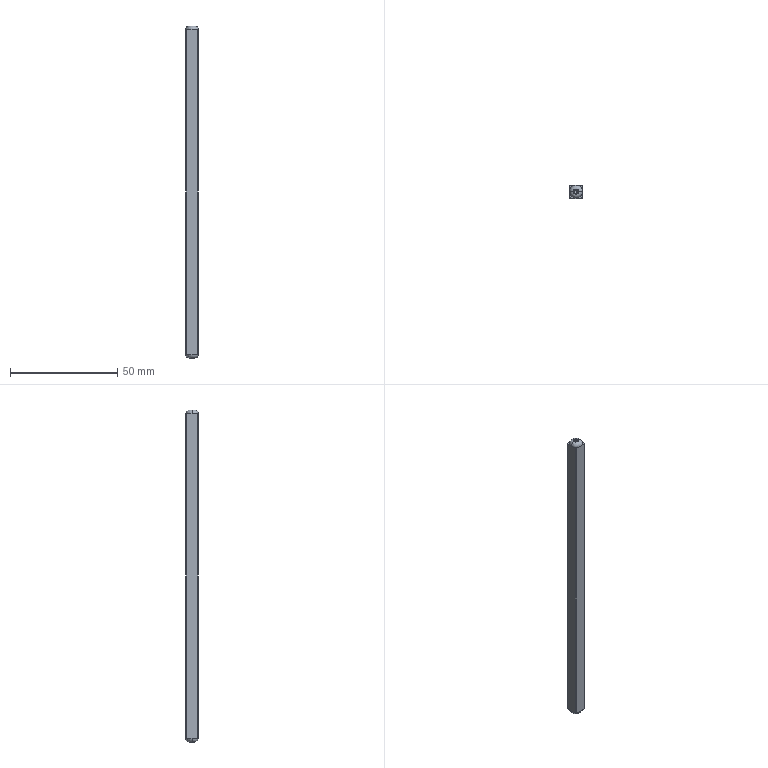Part | NX | features BREP 1 | 1 solid | 34 faces | box 6 x 6 x 155 mm | volume 5484 mm3 | plane 14 | cone 8 | cylinder 8 | torus 4 | commonest cylinder face diameters 1.5 x4 8 x4
STEP:
#1=CARTESIAN_POINT('',(0.75,0.,-77.25));
#2=VERTEX_POINT('',#1);
#3=CARTESIAN_POINT('',(1.,0.,-77.5));
#4=VERTEX_POINT('',#3);
#5=CARTESIAN_POINT('',(1.,0.,-77.5));
#6=DIRECTION('',(0.7071,0.,-0.7071));
#7=VECTOR('',#6,1000.);
#8=LINE('',#5,#7);
#9=EDGE_CURVE('',#2,#4,#8,.T.);
#10=ORIENTED_EDGE('',*,*,#9,.F.);
#11=CARTESIAN_POINT('',(-0.75,0.,-77.25));
#12=VERTEX_POINT('',#11);
#13=CARTESIAN_POINT('',(0.,0.,-77.25));
#14=DIRECTION('',(0.,0.,-1.));
#15=DIRECTION('',(-1.,0.,0.));
#16=AXIS2_PLACEMENT_3D('',#13,#14,#15);
#17=CIRCLE('',#16,0.75);
#18=EDGE_CURVE('',#12,#2,#17,.T.);
#19=ORIENTED_EDGE('',*,*,#18,.F.);
#20=CARTESIAN_POINT('',(-1.,0.,-77.5));
#21=VERTEX_POINT('',#20);
#22=CARTESIAN_POINT('',(-1.,0.,-77.5));
#23=DIRECTION('',(-0.7071,0.,-0.7071));
#24=VECTOR('',#23,1000.);
#25=LINE('',#22,#24);
#26=EDGE_CURVE('',#12,#21,#25,.T.);
#27=ORIENTED_EDGE('',*,*,#26,.T.);
#28=CARTESIAN_POINT('',(0.,0.,-77.5));
#29=DIRECTION('',(0.,0.,-1.));
#30=DIRECTION('',(-1.,0.,0.));
#31=AXIS2_PLACEMENT_3D('',#28,#29,#30);
#32=CIRCLE('',#31,1.);
#33=EDGE_CURVE('',#21,#4,#32,.T.);
#34=ORIENTED_EDGE('',*,*,#33,.T.);
#35=EDGE_LOOP('',(#10,#19,#27,#34));
#36=FACE_BOUND('',#35,.T.);
#37=CARTESIAN_POINT('',(0.,0.,-77.5));
#38=DIRECTION('',(0.,0.,-1.));
#39=DIRECTION('',(-1.,0.,0.));
#40=AXIS2_PLACEMENT_3D('',#37,#38,#39);
#41=CONICAL_SURFACE('',#40,1.,0.7854);
#42=ADVANCED_FACE('',(#36),#41,.F.);
#43=CARTESIAN_POINT('',(0.75,0.,-74.5));
#44=VERTEX_POINT('',#43);
#45=CARTESIAN_POINT('',(0.75,0.,-77.5));
#46=DIRECTION('',(0.,0.,-1.));
#47=VECTOR('',#46,1000.);
#48=LINE('',#45,#47);
#49=EDGE_CURVE('',#44,#2,#48,.T.);
#50=ORIENTED_EDGE('',*,*,#49,.F.);
#51=CARTESIAN_POINT('',(-0.75,0.,-74.5));
#52=VERTEX_POINT('',#51);
#53=CARTESIAN_POINT('',(0.,0.,-74.5));
#54=DIRECTION('',(0.,0.,-1.));
#55=DIRECTION('',(-1.,0.,0.));
#56=AXIS2_PLACEMENT_3D('',#53,#54,#55);
#57=CIRCLE('',#56,0.75);
#58=EDGE_CURVE('',#52,#44,#57,.T.);
#59=ORIENTED_EDGE('',*,*,#58,.F.);
#60=CARTESIAN_POINT('',(-0.75,0.,-77.5));
#61=DIRECTION('',(0.,0.,-1.));
#62=VECTOR('',#61,1000.);
#63=LINE('',#60,#62);
#64=EDGE_CURVE('',#52,#12,#63,.T.);
#65=ORIENTED_EDGE('',*,*,#64,.T.);
#66=ORIENTED_EDGE('',*,*,#18,.T.);
#67=EDGE_LOOP('',(#50,#59,#65,#66));
#68=FACE_BOUND('',#67,.T.);
#69=CARTESIAN_POINT('',(0.,0.,-77.5));
#70=DIRECTION('',(0.,0.,-1.));
#71=DIRECTION('',(-1.,0.,0.));
#72=AXIS2_PLACEMENT_3D('',#69,#70,#71);
#73=CYLINDRICAL_SURFACE('',#72,0.75);
#74=ADVANCED_FACE('',(#68),#73,.F.);
#75=CARTESIAN_POINT('',(0.,0.,-74.049));
#76=VERTEX_POINT('',#75);
#77=CARTESIAN_POINT('',(0.75,0.,-74.5));
#78=DIRECTION('',(0.8572,0.,-0.515));
#79=VECTOR('',#78,1000.);
#80=LINE('',#77,#79);
#81=EDGE_CURVE('',#44,#76,#80,.F.);
#82=ORIENTED_EDGE('',*,*,#81,.T.);
#83=CARTESIAN_POINT('',(-0.75,0.,-74.5));
#84=DIRECTION('',(-0.8572,0.,-0.515));
#85=VECTOR('',#84,1000.);
#86=LINE('',#83,#85);
#87=EDGE_CURVE('',#52,#76,#86,.F.);
#88=ORIENTED_EDGE('',*,*,#87,.F.);
#89=ORIENTED_EDGE('',*,*,#58,.T.);
#90=EDGE_LOOP('',(#82,#88,#89));
#91=FACE_BOUND('',#90,.T.);
#92=CARTESIAN_POINT('',(0.,0.,-74.5));
#93=DIRECTION('',(0.,0.,-1.));
#94=DIRECTION('',(-1.,0.,0.));
#95=AXIS2_PLACEMENT_3D('',#92,#93,#94);
#96=CONICAL_SURFACE('',#95,0.75,1.03);
#97=ADVANCED_FACE('',(#91),#96,.F.);
#98=CARTESIAN_POINT('',(-1.,0.,77.5));
#99=VERTEX_POINT('',#98);
#100=CARTESIAN_POINT('',(-0.75,0.,77.25));
#101=VERTEX_POINT('',#100);
#102=CARTESIAN_POINT('',(-1.,0.,77.5));
#103=DIRECTION('',(-0.7071,0.,0.7071));
#104=VECTOR('',#103,1000.);
#105=LINE('',#102,#104);
#106=EDGE_CURVE('',#99,#101,#105,.F.);
#107=ORIENTED_EDGE('',*,*,#106,.T.);
#108=CARTESIAN_POINT('',(0.75,0.,77.25));
#109=VERTEX_POINT('',#108);
#110=CARTESIAN_POINT('',(0.,0.,77.25));
#111=DIRECTION('',(0.,0.,1.));
#112=DIRECTION('',(1.,0.,0.));
#113=AXIS2_PLACEMENT_3D('',#110,#111,#112);
#114=CIRCLE('',#113,0.75);
#115=EDGE_CURVE('',#109,#101,#114,.T.);
#116=ORIENTED_EDGE('',*,*,#115,.F.);
#117=CARTESIAN_POINT('',(1.,0.,77.5));
#118=VERTEX_POINT('',#117);
#119=CARTESIAN_POINT('',(1.,0.,77.5));
#120=DIRECTION('',(0.7071,0.,0.7071));
#121=VECTOR('',#120,1000.);
#122=LINE('',#119,#121);
#123=EDGE_CURVE('',#118,#109,#122,.F.);
#124=ORIENTED_EDGE('',*,*,#123,.F.);
#125=CARTESIAN_POINT('',(0.,0.,77.5));
#126=DIRECTION('',(0.,0.,1.));
#127=DIRECTION('',(1.,0.,0.));
#128=AXIS2_PLACEMENT_3D('',#125,#126,#127);
#129=CIRCLE('',#128,1.);
#130=EDGE_CURVE('',#118,#99,#129,.T.);
#131=ORIENTED_EDGE('',*,*,#130,.T.);
#132=EDGE_LOOP('',(#107,#116,#124,#131));
#133=FACE_BOUND('',#132,.T.);
#134=CARTESIAN_POINT('',(0.,0.,77.5));
#135=DIRECTION('',(0.,0.,1.));
#136=DIRECTION('',(1.,0.,0.));
#137=AXIS2_PLACEMENT_3D('',#134,#135,#136);
#138=CONICAL_SURFACE('',#137,1.,0.7854);
#139=ADVANCED_FACE('',(#133),#138,.F.);
#140=CARTESIAN_POINT('',(-0.75,0.,74.5));
#141=VERTEX_POINT('',#140);
#142=CARTESIAN_POINT('',(-0.75,0.,77.5));
#143=DIRECTION('',(0.,0.,1.));
#144=VECTOR('',#143,1000.);
#145=LINE('',#142,#144);
#146=EDGE_CURVE('',#101,#141,#145,.F.);
#147=ORIENTED_EDGE('',*,*,#146,.T.);
#148=CARTESIAN_POINT('',(0.75,0.,74.5));
#149=VERTEX_POINT('',#148);
#150=CARTESIAN_POINT('',(0.,0.,74.5));
#151=DIRECTION('',(0.,0.,1.));
#152=DIRECTION('',(1.,0.,0.));
#153=AXIS2_PLACEMENT_3D('',#150,#151,#152);
#154=CIRCLE('',#153,0.75);
#155=EDGE_CURVE('',#149,#141,#154,.T.);
#156=ORIENTED_EDGE('',*,*,#155,.F.);
#157=CARTESIAN_POINT('',(0.75,0.,77.5));
#158=DIRECTION('',(0.,0.,1.));
#159=VECTOR('',#158,1000.);
#160=LINE('',#157,#159);
#161=EDGE_CURVE('',#109,#149,#160,.F.);
#162=ORIENTED_EDGE('',*,*,#161,.F.);
#163=ORIENTED_EDGE('',*,*,#115,.T.);
#164=EDGE_LOOP('',(#147,#156,#162,#163));
#165=FACE_BOUND('',#164,.T.);
#166=CARTESIAN_POINT('',(0.,0.,77.5));
#167=DIRECTION('',(0.,0.,1.));
#168=DIRECTION('',(1.,0.,0.));
#169=AXIS2_PLACEMENT_3D('',#166,#167,#168);
#170=CYLINDRICAL_SURFACE('',#169,0.75);
#171=ADVANCED_FACE('',(#165),#170,.F.);
#172=CARTESIAN_POINT('',(0.,0.,74.049));
#173=VERTEX_POINT('',#172);
#174=CARTESIAN_POINT('',(-0.75,0.,74.5));
#175=DIRECTION('',(-0.8572,0.,0.515));
#176=VECTOR('',#175,1000.);
#177=LINE('',#174,#176);
#178=EDGE_CURVE('',#173,#141,#177,.T.);
#179=ORIENTED_EDGE('',*,*,#178,.F.);
#180=CARTESIAN_POINT('',(0.75,0.,74.5));
#181=DIRECTION('',(0.8572,0.,0.515));
#182=VECTOR('',#181,1000.);
#183=LINE('',#180,#182);
#184=EDGE_CURVE('',#173,#149,#183,.T.);
#185=ORIENTED_EDGE('',*,*,#184,.T.);
#186=ORIENTED_EDGE('',*,*,#155,.T.);
#187=EDGE_LOOP('',(#179,#185,#186));
#188=FACE_BOUND('',#187,.T.);
#189=CARTESIAN_POINT('',(0.,0.,74.5));
#190=DIRECTION('',(0.,0.,1.));
#191=DIRECTION('',(1.,0.,0.));
#192=AXIS2_PLACEMENT_3D('',#189,#190,#191);
#193=CONICAL_SURFACE('',#192,0.75,1.03);
#194=ADVANCED_FACE('',(#188),#193,.F.);
#195=CARTESIAN_POINT('',(-1.25,0.,-77.5));
#196=VERTEX_POINT('',#195);
#197=CARTESIAN_POINT('',(1.25,0.,-77.5));
#198=VERTEX_POINT('',#197);
#199=CARTESIAN_POINT('',(0.,0.,-77.5));
#200=DIRECTION('',(0.,0.,-1.));
#201=DIRECTION('',(-1.,0.,0.));
#202=AXIS2_PLACEMENT_3D('',#199,#200,#201);
#203=CIRCLE('',#202,1.25);
#204=EDGE_CURVE('',#196,#198,#203,.T.);
#205=ORIENTED_EDGE('',*,*,#204,.T.);
#206=CARTESIAN_POINT('',(0.,0.,-77.5));
#207=DIRECTION('',(0.,0.,-1.));
#208=DIRECTION('',(-1.,0.,0.));
#209=AXIS2_PLACEMENT_3D('',#206,#207,#208);
#210=CIRCLE('',#209,1.25);
#211=EDGE_CURVE('',#198,#196,#210,.T.);
#212=ORIENTED_EDGE('',*,*,#211,.T.);
#213=EDGE_LOOP('',(#205,#212));
#214=FACE_BOUND('',#213,.T.);
#215=ORIENTED_EDGE('',*,*,#33,.F.);
#216=CARTESIAN_POINT('',(0.,0.,-77.5));
#217=DIRECTION('',(0.,0.,-1.));
#218=DIRECTION('',(-1.,0.,0.));
#219=AXIS2_PLACEMENT_3D('',#216,#217,#218);
#220=CIRCLE('',#219,1.);
#221=EDGE_CURVE('',#4,#21,#220,.T.);
#222=ORIENTED_EDGE('',*,*,#221,.F.);
#223=EDGE_LOOP('',(#215,#222));
#224=FACE_BOUND('',#223,.T.);
#225=CARTESIAN_POINT('',(0.,0.,-77.5));
#226=DIRECTION('',(0.,0.,1.));
#227=DIRECTION('',(1.,0.,0.));
#228=AXIS2_PLACEMENT_3D('',#225,#226,#227);
#229=PLANE('',#228);
#230=ADVANCED_FACE('',(#214,#224),#229,.F.);
#231=CARTESIAN_POINT('',(3.,0.,-75.75));
#232=VERTEX_POINT('',#231);
#233=CARTESIAN_POINT('',(1.25,0.,-75.75));
#234=DIRECTION('',(0.,-1.,0.));
#235=DIRECTION('',(1.,0.,0.));
#236=AXIS2_PLACEMENT_3D('',#233,#234,#235);
#237=CIRCLE('',#236,1.75);
#238=EDGE_CURVE('',#198,#232,#237,.T.);
#239=ORIENTED_EDGE('',*,*,#238,.F.);
#240=ORIENTED_EDGE('',*,*,#204,.F.);
#241=CARTESIAN_POINT('',(-3.,0.,-75.75));
#242=VERTEX_POINT('',#241);
#243=CARTESIAN_POINT('',(-1.25,0.,-75.75));
#244=DIRECTION('',(0.,1.,0.));
#245=DIRECTION('',(0.,0.,1.));
#246=AXIS2_PLACEMENT_3D('',#243,#244,#245);
#247=CIRCLE('',#246,1.75);
#248=EDGE_CURVE('',#196,#242,#247,.T.);
#249=ORIENTED_EDGE('',*,*,#248,.T.);
#250=CARTESIAN_POINT('',(0.,3.,-75.75));
#251=VERTEX_POINT('',#250);
#252=CARTESIAN_POINT('',(0.,0.,-75.75));
#253=DIRECTION('',(0.,0.,-1.));
#254=DIRECTION('',(-1.,0.,0.));
#255=AXIS2_PLACEMENT_3D('',#252,#253,#254);
#256=CIRCLE('',#255,3.);
#257=EDGE_CURVE('',#242,#251,#256,.T.);
#258=ORIENTED_EDGE('',*,*,#257,.T.);
#259=CARTESIAN_POINT('',(0.,0.,-75.75));
#260=DIRECTION('',(0.,0.,-1.));
#261=DIRECTION('',(-1.,0.,0.));
#262=AXIS2_PLACEMENT_3D('',#259,#260,#261);
#263=CIRCLE('',#262,3.);
#264=EDGE_CURVE('',#251,#232,#263,.T.);
#265=ORIENTED_EDGE('',*,*,#264,.T.);
#266=EDGE_LOOP('',(#239,#240,#249,#258,#265));
#267=FACE_BOUND('',#266,.T.);
#268=CARTESIAN_POINT('',(0.,0.,-75.75));
#269=DIRECTION('',(0.,0.,1.));
#270=DIRECTION('',(-1.,0.,0.));
#271=AXIS2_PLACEMENT_3D('',#268,#269,#270);
#272=DEGENERATE_TOROIDAL_SURFACE('',#271,1.25,1.75,.T.);
#273=ADVANCED_FACE('',(#267),#272,.T.);
#274=CARTESIAN_POINT('',(-2.646,3.,-75.75));
#275=VERTEX_POINT('',#274);
#276=CARTESIAN_POINT('',(-2.646,3.,-75.75));
#277=DIRECTION('',(1.,0.,0.));
#278=VECTOR('',#277,1000.);
#279=LINE('',#276,#278);
#280=EDGE_CURVE('',#275,#251,#279,.T.);
#281=ORIENTED_EDGE('',*,*,#280,.T.);
#282=ORIENTED_EDGE('',*,*,#257,.F.);
#283=CARTESIAN_POINT('',(-3.,2.646,-75.75));
#284=VERTEX_POINT('',#283);
#285=CARTESIAN_POINT('',(-3.,-2.646,-75.75));
#286=DIRECTION('',(0.,1.,0.));
#287=VECTOR('',#286,1000.);
#288=LINE('',#285,#287);
#289=EDGE_CURVE('',#242,#284,#288,.T.);
#290=ORIENTED_EDGE('',*,*,#289,.T.);
#291=CARTESIAN_POINT('',(0.,0.,-75.75));
#292=DIRECTION('',(0.,0.,-1.));
#293=DIRECTION('',(-1.,0.,0.));
#294=AXIS2_PLACEMENT_3D('',#291,#292,#293);
#295=CIRCLE('',#294,4.);
#296=EDGE_CURVE('',#284,#275,#295,.T.);
#297=ORIENTED_EDGE('',*,*,#296,.T.);
#298=EDGE_LOOP('',(#281,#282,#290,#297));
#299=FACE_BOUND('',#298,.T.);
#300=CARTESIAN_POINT('',(3.,0.,-75.75));
#301=DIRECTION('',(0.,0.,-1.));
#302=DIRECTION('',(1.,0.,0.));
#303=AXIS2_PLACEMENT_3D('',#300,#301,#302);
#304=PLANE('',#303);
#305=ADVANCED_FACE('',(#299),#304,.T.);
#306=CARTESIAN_POINT('',(3.,2.646,-75.75));
#307=VERTEX_POINT('',#306);
#308=CARTESIAN_POINT('',(3.,-2.646,-75.75));
#309=DIRECTION('',(0.,-1.,0.));
#310=VECTOR('',#309,1000.);
#311=LINE('',#308,#310);
#312=EDGE_CURVE('',#307,#232,#311,.T.);
#313=ORIENTED_EDGE('',*,*,#312,.T.);
#314=ORIENTED_EDGE('',*,*,#264,.F.);
#315=CARTESIAN_POINT('',(2.646,3.,-75.75));
#316=VERTEX_POINT('',#315);
#317=CARTESIAN_POINT('',(-2.646,3.,-75.75));
#318=DIRECTION('',(1.,0.,0.));
#319=VECTOR('',#318,1000.);
#320=LINE('',#317,#319);
#321=EDGE_CURVE('',#251,#316,#320,.T.);
#322=ORIENTED_EDGE('',*,*,#321,.T.);
#323=CARTESIAN_POINT('',(0.,0.,-75.75));
#324=DIRECTION('',(0.,0.,-1.));
#325=DIRECTION('',(-1.,0.,0.));
#326=AXIS2_PLACEMENT_3D('',#323,#324,#325);
#327=CIRCLE('',#326,4.);
#328=EDGE_CURVE('',#316,#307,#327,.T.);
#329=ORIENTED_EDGE('',*,*,#328,.T.);
#330=EDGE_LOOP('',(#313,#314,#322,#329));
#331=FACE_BOUND('',#330,.T.);
#332=CARTESIAN_POINT('',(3.,0.,-75.75));
#333=DIRECTION('',(0.,0.,-1.));
#334=DIRECTION('',(1.,0.,0.));
#335=AXIS2_PLACEMENT_3D('',#332,#333,#334);
#336=PLANE('',#335);
#337=ADVANCED_FACE('',(#331),#336,.T.);
#338=CARTESIAN_POINT('',(0.,-3.,-75.75));
#339=VERTEX_POINT('',#338);
#340=CARTESIAN_POINT('',(-2.646,-3.,-75.75));
#341=VERTEX_POINT('',#340);
#342=CARTESIAN_POINT('',(-2.646,-3.,-75.75));
#343=DIRECTION('',(-1.,0.,0.));
#344=VECTOR('',#343,1000.);
#345=LINE('',#342,#344);
#346=EDGE_CURVE('',#339,#341,#345,.T.);
#347=ORIENTED_EDGE('',*,*,#346,.T.);
#348=CARTESIAN_POINT('',(-3.,-2.646,-75.75));
#349=VERTEX_POINT('',#348);
#350=CARTESIAN_POINT('',(0.,0.,-75.75));
#351=DIRECTION('',(0.,0.,-1.));
#352=DIRECTION('',(-1.,0.,0.));
#353=AXIS2_PLACEMENT_3D('',#350,#351,#352);
#354=CIRCLE('',#353,4.);
#355=EDGE_CURVE('',#341,#349,#354,.T.);
#356=ORIENTED_EDGE('',*,*,#355,.T.);
#357=CARTESIAN_POINT('',(-3.,-2.646,-75.75));
#358=DIRECTION('',(0.,1.,0.));
#359=VECTOR('',#358,1000.);
#360=LINE('',#357,#359);
#361=EDGE_CURVE('',#349,#242,#360,.T.);
#362=ORIENTED_EDGE('',*,*,#361,.T.);
#363=CARTESIAN_POINT('',(0.,0.,-75.75));
#364=DIRECTION('',(0.,0.,-1.));
#365=DIRECTION('',(-1.,0.,0.));
#366=AXIS2_PLACEMENT_3D('',#363,#364,#365);
#367=CIRCLE('',#366,3.);
#368=EDGE_CURVE('',#339,#242,#367,.T.);
#369=ORIENTED_EDGE('',*,*,#368,.F.);
#370=EDGE_LOOP('',(#347,#356,#362,#369));
#371=FACE_BOUND('',#370,.T.);
#372=CARTESIAN_POINT('',(3.,0.,-75.75));
#373=DIRECTION('',(0.,0.,-1.));
#374=DIRECTION('',(1.,0.,0.));
#375=AXIS2_PLACEMENT_3D('',#372,#373,#374);
#376=PLANE('',#375);
#377=ADVANCED_FACE('',(#371),#376,.T.);
#378=CARTESIAN_POINT('',(3.,-2.646,-75.75));
#379=VERTEX_POINT('',#378);
#380=CARTESIAN_POINT('',(2.646,-3.,-75.75));
#381=VERTEX_POINT('',#380);
#382=CARTESIAN_POINT('',(0.,0.,-75.75));
#383=DIRECTION('',(0.,0.,-1.));
#384=DIRECTION('',(-1.,0.,0.));
#385=AXIS2_PLACEMENT_3D('',#382,#383,#384);
#386=CIRCLE('',#385,4.);
#387=EDGE_CURVE('',#379,#381,#386,.T.);
#388=ORIENTED_EDGE('',*,*,#387,.T.);
#389=CARTESIAN_POINT('',(-2.646,-3.,-75.75));
#390=DIRECTION('',(-1.,0.,0.));
#391=VECTOR('',#390,1000.);
#392=LINE('',#389,#391);
#393=EDGE_CURVE('',#381,#339,#392,.T.);
#394=ORIENTED_EDGE('',*,*,#393,.T.);
#395=CARTESIAN_POINT('',(0.,0.,-75.75));
#396=DIRECTION('',(0.,0.,-1.));
#397=DIRECTION('',(-1.,0.,0.));
#398=AXIS2_PLACEMENT_3D('',#395,#396,#397);
#399=CIRCLE('',#398,3.);
#400=EDGE_CURVE('',#232,#339,#399,.T.);
#401=ORIENTED_EDGE('',*,*,#400,.F.);
#402=CARTESIAN_POINT('',(3.,-2.646,-75.75));
#403=DIRECTION('',(0.,-1.,0.));
#404=VECTOR('',#403,1000.);
#405=LINE('',#402,#404);
#406=EDGE_CURVE('',#232,#379,#405,.T.);
#407=ORIENTED_EDGE('',*,*,#406,.T.);
#408=EDGE_LOOP('',(#388,#394,#401,#407));
#409=FACE_BOUND('',#408,.T.);
#410=CARTESIAN_POINT('',(3.,0.,-75.75));
#411=DIRECTION('',(0.,0.,-1.));
#412=DIRECTION('',(1.,0.,0.));
#413=AXIS2_PLACEMENT_3D('',#410,#411,#412);
#414=PLANE('',#413);
#415=ADVANCED_FACE('',(#409),#414,.T.);
#416=CARTESIAN_POINT('',(-1.25,0.,77.5));
#417=VERTEX_POINT('',#416);
#418=CARTESIAN_POINT('',(1.25,0.,77.5));
#419=VERTEX_POINT('',#418);
#420=CARTESIAN_POINT('',(0.,0.,77.5));
#421=DIRECTION('',(0.,0.,-1.));
#422=DIRECTION('',(-1.,0.,0.));
#423=AXIS2_PLACEMENT_3D('',#420,#421,#422);
#424=CIRCLE('',#423,1.25);
#425=EDGE_CURVE('',#417,#419,#424,.T.);
#426=ORIENTED_EDGE('',*,*,#425,.F.);
#427=CARTESIAN_POINT('',(0.,0.,77.5));
#428=DIRECTION('',(0.,0.,-1.));
#429=DIRECTION('',(-1.,0.,0.));
#430=AXIS2_PLACEMENT_3D('',#427,#428,#429);
#431=CIRCLE('',#430,1.25);
#432=EDGE_CURVE('',#419,#417,#431,.T.);
#433=ORIENTED_EDGE('',*,*,#432,.F.);
#434=EDGE_LOOP('',(#426,#433));
#435=FACE_BOUND('',#434,.T.);
#436=ORIENTED_EDGE('',*,*,#130,.F.);
#437=CARTESIAN_POINT('',(0.,0.,77.5));
#438=DIRECTION('',(0.,0.,1.));
#439=DIRECTION('',(1.,0.,0.));
#440=AXIS2_PLACEMENT_3D('',#437,#438,#439);
#441=CIRCLE('',#440,1.);
#442=EDGE_CURVE('',#99,#118,#441,.T.);
#443=ORIENTED_EDGE('',*,*,#442,.F.);
#444=EDGE_LOOP('',(#436,#443));
#445=FACE_BOUND('',#444,.T.);
#446=CARTESIAN_POINT('',(0.,0.,77.5));
#447=DIRECTION('',(0.,0.,1.));
#448=DIRECTION('',(1.,0.,0.));
#449=AXIS2_PLACEMENT_3D('',#446,#447,#448);
#450=PLANE('',#449);
#451=ADVANCED_FACE('',(#435,#445),#450,.T.);
#452=CARTESIAN_POINT('',(3.,0.,75.75));
#453=VERTEX_POINT('',#452);
#454=CARTESIAN_POINT('',(1.25,0.,75.75));
#455=DIRECTION('',(0.,1.,0.));
#456=DIRECTION('',(-1.,0.,0.));
#457=AXIS2_PLACEMENT_3D('',#454,#455,#456);
#458=CIRCLE('',#457,1.75);
#459=EDGE_CURVE('',#419,#453,#458,.T.);
#460=ORIENTED_EDGE('',*,*,#459,.F.);
#461=ORIENTED_EDGE('',*,*,#432,.T.);
#462=CARTESIAN_POINT('',(-3.,0.,75.75));
#463=VERTEX_POINT('',#462);
#464=CARTESIAN_POINT('',(-1.25,0.,75.75));
#465=DIRECTION('',(0.,-1.,0.));
#466=DIRECTION('',(0.,0.,-1.));
#467=AXIS2_PLACEMENT_3D('',#464,#465,#466);
#468=CIRCLE('',#467,1.75);
#469=EDGE_CURVE('',#417,#463,#468,.T.);
#470=ORIENTED_EDGE('',*,*,#469,.T.);
#471=CARTESIAN_POINT('',(0.,-3.,75.75));
#472=VERTEX_POINT('',#471);
#473=CARTESIAN_POINT('',(0.,0.,75.75));
#474=DIRECTION('',(0.,0.,-1.));
#475=DIRECTION('',(-1.,0.,0.));
#476=AXIS2_PLACEMENT_3D('',#473,#474,#475);
#477=CIRCLE('',#476,3.);
#478=EDGE_CURVE('',#472,#463,#477,.T.);
#479=ORIENTED_EDGE('',*,*,#478,.F.);
#480=CARTESIAN_POINT('',(0.,0.,75.75));
#481=DIRECTION('',(0.,0.,-1.));
#482=DIRECTION('',(-1.,0.,0.));
#483=AXIS2_PLACEMENT_3D('',#480,#481,#482);
#484=CIRCLE('',#483,3.);
#485=EDGE_CURVE('',#453,#472,#484,.T.);
#486=ORIENTED_EDGE('',*,*,#485,.F.);
#487=EDGE_LOOP('',(#460,#461,#470,#479,#486));
#488=FACE_BOUND('',#487,.T.);
#489=CARTESIAN_POINT('',(0.,0.,75.75));
#490=DIRECTION('',(0.,0.,-1.));
#491=DIRECTION('',(-1.,0.,0.));
#492=AXIS2_PLACEMENT_3D('',#489,#490,#491);
#493=DEGENERATE_TOROIDAL_SURFACE('',#492,1.25,1.75,.T.);
#494=ADVANCED_FACE('',(#488),#493,.T.);
#495=CARTESIAN_POINT('',(0.,3.,75.75));
#496=VERTEX_POINT('',#495);
#497=CARTESIAN_POINT('',(-2.646,3.,75.75));
#498=VERTEX_POINT('',#497);
#499=CARTESIAN_POINT('',(-2.646,3.,75.75));
#500=DIRECTION('',(-1.,0.,0.));
#501=VECTOR('',#500,1000.);
#502=LINE('',#499,#501);
#503=EDGE_CURVE('',#496,#498,#502,.T.);
#504=ORIENTED_EDGE('',*,*,#503,.T.);
#505=CARTESIAN_POINT('',(-3.,2.646,75.75));
#506=VERTEX_POINT('',#505);
#507=CARTESIAN_POINT('',(0.,0.,75.75));
#508=DIRECTION('',(0.,0.,1.));
#509=DIRECTION('',(1.,0.,0.));
#510=AXIS2_PLACEMENT_3D('',#507,#508,#509);
#511=CIRCLE('',#510,4.);
#512=EDGE_CURVE('',#498,#506,#511,.T.);
#513=ORIENTED_EDGE('',*,*,#512,.T.);
#514=CARTESIAN_POINT('',(-3.,-2.646,75.75));
#515=DIRECTION('',(0.,-1.,0.));
#516=VECTOR('',#515,1000.);
#517=LINE('',#514,#516);
#518=EDGE_CURVE('',#506,#463,#517,.T.);
#519=ORIENTED_EDGE('',*,*,#518,.T.);
#520=CARTESIAN_POINT('',(0.,0.,75.75));
#521=DIRECTION('',(0.,0.,-1.));
#522=DIRECTION('',(-1.,0.,0.));
#523=AXIS2_PLACEMENT_3D('',#520,#521,#522);
#524=CIRCLE('',#523,3.);
#525=EDGE_CURVE('',#463,#496,#524,.T.);
#526=ORIENTED_EDGE('',*,*,#525,.T.);
#527=EDGE_LOOP('',(#504,#513,#519,#526));
#528=FACE_BOUND('',#527,.T.);
#529=CARTESIAN_POINT('',(3.,0.,75.75));
#530=DIRECTION('',(0.,0.,1.));
#531=DIRECTION('',(1.,0.,0.));
#532=AXIS2_PLACEMENT_3D('',#529,#530,#531);
#533=PLANE('',#532);
#534=ADVANCED_FACE('',(#528),#533,.T.);
#535=CARTESIAN_POINT('',(3.,2.646,75.75));
#536=VERTEX_POINT('',#535);
#537=CARTESIAN_POINT('',(3.,-2.646,75.75));
#538=DIRECTION('',(0.,1.,0.));
#539=VECTOR('',#538,1000.);
#540=LINE('',#537,#539);
#541=EDGE_CURVE('',#453,#536,#540,.T.);
#542=ORIENTED_EDGE('',*,*,#541,.T.);
#543=CARTESIAN_POINT('',(2.646,3.,75.75));
#544=VERTEX_POINT('',#543);
#545=CARTESIAN_POINT('',(0.,0.,75.75));
#546=DIRECTION('',(0.,0.,1.));
#547=DIRECTION('',(1.,0.,0.));
#548=AXIS2_PLACEMENT_3D('',#545,#546,#547);
#549=CIRCLE('',#548,4.);
#550=EDGE_CURVE('',#536,#544,#549,.T.);
#551=ORIENTED_EDGE('',*,*,#550,.T.);
#552=CARTESIAN_POINT('',(-2.646,3.,75.75));
#553=DIRECTION('',(-1.,0.,0.));
#554=VECTOR('',#553,1000.);
#555=LINE('',#552,#554);
#556=EDGE_CURVE('',#544,#496,#555,.T.);
#557=ORIENTED_EDGE('',*,*,#556,.T.);
#558=CARTESIAN_POINT('',(0.,0.,75.75));
#559=DIRECTION('',(0.,0.,-1.));
#560=DIRECTION('',(-1.,0.,0.));
#561=AXIS2_PLACEMENT_3D('',#558,#559,#560);
#562=CIRCLE('',#561,3.);
#563=EDGE_CURVE('',#496,#453,#562,.T.);
#564=ORIENTED_EDGE('',*,*,#563,.T.);
#565=EDGE_LOOP('',(#542,#551,#557,#564));
#566=FACE_BOUND('',#565,.T.);
#567=CARTESIAN_POINT('',(3.,0.,75.75));
#568=DIRECTION('',(0.,0.,1.));
#569=DIRECTION('',(1.,0.,0.));
#570=AXIS2_PLACEMENT_3D('',#567,#568,#569);
#571=PLANE('',#570);
#572=ADVANCED_FACE('',(#566),#571,.T.);
#573=CARTESIAN_POINT('',(2.646,-3.,75.75));
#574=VERTEX_POINT('',#573);
#575=CARTESIAN_POINT('',(-2.646,-3.,75.75));
#576=DIRECTION('',(1.,0.,0.));
#577=VECTOR('',#576,1000.);
#578=LINE('',#575,#577);
#579=EDGE_CURVE('',#472,#574,#578,.T.);
#580=ORIENTED_EDGE('',*,*,#579,.T.);
#581=CARTESIAN_POINT('',(3.,-2.646,75.75));
#582=VERTEX_POINT('',#581);
#583=CARTESIAN_POINT('',(0.,0.,75.75));
#584=DIRECTION('',(0.,0.,1.));
#585=DIRECTION('',(1.,0.,0.));
#586=AXIS2_PLACEMENT_3D('',#583,#584,#585);
#587=CIRCLE('',#586,4.);
#588=EDGE_CURVE('',#574,#582,#587,.T.);
#589=ORIENTED_EDGE('',*,*,#588,.T.);
#590=CARTESIAN_POINT('',(3.,-2.646,75.75));
#591=DIRECTION('',(0.,1.,0.));
#592=VECTOR('',#591,1000.);
#593=LINE('',#590,#592);
#594=EDGE_CURVE('',#582,#453,#593,.T.);
#595=ORIENTED_EDGE('',*,*,#594,.T.);
#596=ORIENTED_EDGE('',*,*,#485,.T.);
#597=EDGE_LOOP('',(#580,#589,#595,#596));
#598=FACE_BOUND('',#597,.T.);
#599=CARTESIAN_POINT('',(3.,0.,75.75));
#600=DIRECTION('',(0.,0.,1.));
#601=DIRECTION('',(1.,0.,0.));
#602=AXIS2_PLACEMENT_3D('',#599,#600,#601);
#603=PLANE('',#602);
#604=ADVANCED_FACE('',(#598),#603,.T.);
#605=CARTESIAN_POINT('',(-3.,-2.646,75.75));
#606=VERTEX_POINT('',#605);
#607=CARTESIAN_POINT('',(-2.646,-3.,75.75));
#608=VERTEX_POINT('',#607);
#609=CARTESIAN_POINT('',(0.,0.,75.75));
#610=DIRECTION('',(0.,0.,1.));
#611=DIRECTION('',(1.,0.,0.));
#612=AXIS2_PLACEMENT_3D('',#609,#610,#611);
#613=CIRCLE('',#612,4.);
#614=EDGE_CURVE('',#606,#608,#613,.T.);
#615=ORIENTED_EDGE('',*,*,#614,.T.);
#616=CARTESIAN_POINT('',(-2.646,-3.,75.75));
#617=DIRECTION('',(1.,0.,0.));
#618=VECTOR('',#617,1000.);
#619=LINE('',#616,#618);
#620=EDGE_CURVE('',#608,#472,#619,.T.);
#621=ORIENTED_EDGE('',*,*,#620,.T.);
#622=ORIENTED_EDGE('',*,*,#478,.T.);
#623=CARTESIAN_POINT('',(-3.,-2.646,75.75));
#624=DIRECTION('',(0.,-1.,0.));
#625=VECTOR('',#624,1000.);
#626=LINE('',#623,#625);
#627=EDGE_CURVE('',#463,#606,#626,.T.);
#628=ORIENTED_EDGE('',*,*,#627,.T.);
#629=EDGE_LOOP('',(#615,#621,#622,#628));
#630=FACE_BOUND('',#629,.T.);
#631=CARTESIAN_POINT('',(3.,0.,75.75));
#632=DIRECTION('',(0.,0.,1.));
#633=DIRECTION('',(1.,0.,0.));
#634=AXIS2_PLACEMENT_3D('',#631,#632,#633);
#635=PLANE('',#634);
#636=ADVANCED_FACE('',(#630),#635,.T.);
#637=ORIENTED_EDGE('',*,*,#361,.F.);
#638=CARTESIAN_POINT('',(-3.,-2.646,77.5));
#639=DIRECTION('',(0.,0.,-1.));
#640=VECTOR('',#639,1000.);
#641=LINE('',#638,#640);
#642=EDGE_CURVE('',#606,#349,#641,.T.);
#643=ORIENTED_EDGE('',*,*,#642,.F.);
#644=ORIENTED_EDGE('',*,*,#627,.F.);
#645=ORIENTED_EDGE('',*,*,#518,.F.);
#646=CARTESIAN_POINT('',(-3.,2.646,77.5));
#647=DIRECTION('',(0.,0.,-1.));
#648=VECTOR('',#647,1000.);
#649=LINE('',#646,#648);
#650=EDGE_CURVE('',#506,#284,#649,.T.);
#651=ORIENTED_EDGE('',*,*,#650,.T.);
#652=ORIENTED_EDGE('',*,*,#289,.F.);
#653=EDGE_LOOP('',(#637,#643,#644,#645,#651,#652));
#654=FACE_BOUND('',#653,.T.);
#655=CARTESIAN_POINT('',(-3.,-2.646,77.5));
#656=DIRECTION('',(1.,0.,0.));
#657=DIRECTION('',(0.,0.,-1.));
#658=AXIS2_PLACEMENT_3D('',#655,#656,#657);
#659=PLANE('',#658);
#660=ADVANCED_FACE('',(#654),#659,.F.);
#661=ORIENTED_EDGE('',*,*,#296,.F.);
#662=ORIENTED_EDGE('',*,*,#650,.F.);
#663=ORIENTED_EDGE('',*,*,#512,.F.);
#664=CARTESIAN_POINT('',(-2.646,3.,77.5));
#665=DIRECTION('',(0.,0.,-1.));
#666=VECTOR('',#665,1000.);
#667=LINE('',#664,#666);
#668=EDGE_CURVE('',#498,#275,#667,.T.);
#669=ORIENTED_EDGE('',*,*,#668,.T.);
#670=EDGE_LOOP('',(#661,#662,#663,#669));
#671=FACE_BOUND('',#670,.T.);
#672=CARTESIAN_POINT('',(0.,0.,77.5));
#673=DIRECTION('',(0.,0.,-1.));
#674=DIRECTION('',(-1.,0.,0.));
#675=AXIS2_PLACEMENT_3D('',#672,#673,#674);
#676=CYLINDRICAL_SURFACE('',#675,4.);
#677=ADVANCED_FACE('',(#671),#676,.T.);
#678=ORIENTED_EDGE('',*,*,#280,.F.);
#679=ORIENTED_EDGE('',*,*,#668,.F.);
#680=ORIENTED_EDGE('',*,*,#503,.F.);
#681=ORIENTED_EDGE('',*,*,#556,.F.);
#682=CARTESIAN_POINT('',(2.646,3.,77.5));
#683=DIRECTION('',(0.,0.,-1.));
#684=VECTOR('',#683,1000.);
#685=LINE('',#682,#684);
#686=EDGE_CURVE('',#544,#316,#685,.T.);
#687=ORIENTED_EDGE('',*,*,#686,.T.);
#688=ORIENTED_EDGE('',*,*,#321,.F.);
#689=EDGE_LOOP('',(#678,#679,#680,#681,#687,#688));
#690=FACE_BOUND('',#689,.T.);
#691=CARTESIAN_POINT('',(-2.646,3.,77.5));
#692=DIRECTION('',(0.,-1.,0.));
#693=DIRECTION('',(0.,0.,-1.));
#694=AXIS2_PLACEMENT_3D('',#691,#692,#693);
#695=PLANE('',#694);
#696=ADVANCED_FACE('',(#690),#695,.F.);
#697=ORIENTED_EDGE('',*,*,#328,.F.);
#698=ORIENTED_EDGE('',*,*,#686,.F.);
#699=ORIENTED_EDGE('',*,*,#550,.F.);
#700=CARTESIAN_POINT('',(3.,2.646,77.5));
#701=DIRECTION('',(0.,0.,-1.));
#702=VECTOR('',#701,1000.);
#703=LINE('',#700,#702);
#704=EDGE_CURVE('',#536,#307,#703,.T.);
#705=ORIENTED_EDGE('',*,*,#704,.T.);
#706=EDGE_LOOP('',(#697,#698,#699,#705));
#707=FACE_BOUND('',#706,.T.);
#708=CARTESIAN_POINT('',(0.,0.,77.5));
#709=DIRECTION('',(0.,0.,-1.));
#710=DIRECTION('',(-1.,0.,0.));
#711=AXIS2_PLACEMENT_3D('',#708,#709,#710);
#712=CYLINDRICAL_SURFACE('',#711,4.);
#713=ADVANCED_FACE('',(#707),#712,.T.);
#714=ORIENTED_EDGE('',*,*,#312,.F.);
#715=ORIENTED_EDGE('',*,*,#704,.F.);
#716=ORIENTED_EDGE('',*,*,#541,.F.);
#717=ORIENTED_EDGE('',*,*,#594,.F.);
#718=CARTESIAN_POINT('',(3.,-2.646,77.5));
#719=DIRECTION('',(0.,0.,-1.));
#720=VECTOR('',#719,1000.);
#721=LINE('',#718,#720);
#722=EDGE_CURVE('',#582,#379,#721,.T.);
#723=ORIENTED_EDGE('',*,*,#722,.T.);
#724=ORIENTED_EDGE('',*,*,#406,.F.);
#725=EDGE_LOOP('',(#714,#715,#716,#717,#723,#724));
#726=FACE_BOUND('',#725,.T.);
#727=CARTESIAN_POINT('',(3.,-2.646,77.5));
#728=DIRECTION('',(-1.,0.,0.));
#729=DIRECTION('',(0.,-1.,0.));
#730=AXIS2_PLACEMENT_3D('',#727,#728,#729);
#731=PLANE('',#730);
#732=ADVANCED_FACE('',(#726),#731,.F.);
#733=ORIENTED_EDGE('',*,*,#387,.F.);
#734=ORIENTED_EDGE('',*,*,#722,.F.);
#735=ORIENTED_EDGE('',*,*,#588,.F.);
#736=CARTESIAN_POINT('',(2.646,-3.,77.5));
#737=DIRECTION('',(0.,0.,-1.));
#738=VECTOR('',#737,1000.);
#739=LINE('',#736,#738);
#740=EDGE_CURVE('',#574,#381,#739,.T.);
#741=ORIENTED_EDGE('',*,*,#740,.T.);
#742=EDGE_LOOP('',(#733,#734,#735,#741));
#743=FACE_BOUND('',#742,.T.);
#744=CARTESIAN_POINT('',(0.,0.,77.5));
#745=DIRECTION('',(0.,0.,-1.));
#746=DIRECTION('',(-1.,0.,0.));
#747=AXIS2_PLACEMENT_3D('',#744,#745,#746);
#748=CYLINDRICAL_SURFACE('',#747,4.);
#749=ADVANCED_FACE('',(#743),#748,.T.);
#750=ORIENTED_EDGE('',*,*,#393,.F.);
#751=ORIENTED_EDGE('',*,*,#740,.F.);
#752=ORIENTED_EDGE('',*,*,#579,.F.);
#753=ORIENTED_EDGE('',*,*,#620,.F.);
#754=CARTESIAN_POINT('',(-2.646,-3.,77.5));
#755=DIRECTION('',(0.,0.,-1.));
#756=VECTOR('',#755,1000.);
#757=LINE('',#754,#756);
#758=EDGE_CURVE('',#608,#341,#757,.T.);
#759=ORIENTED_EDGE('',*,*,#758,.T.);
#760=ORIENTED_EDGE('',*,*,#346,.F.);
#761=EDGE_LOOP('',(#750,#751,#752,#753,#759,#760));
#762=FACE_BOUND('',#761,.T.);
#763=CARTESIAN_POINT('',(-2.646,-3.,77.5));
#764=DIRECTION('',(0.,1.,0.));
#765=DIRECTION('',(0.,0.,1.));
#766=AXIS2_PLACEMENT_3D('',#763,#764,#765);
#767=PLANE('',#766);
#768=ADVANCED_FACE('',(#762),#767,.F.);
#769=ORIENTED_EDGE('',*,*,#355,.F.);
#770=ORIENTED_EDGE('',*,*,#758,.F.);
#771=ORIENTED_EDGE('',*,*,#614,.F.);
#772=ORIENTED_EDGE('',*,*,#642,.T.);
#773=EDGE_LOOP('',(#769,#770,#771,#772));
#774=FACE_BOUND('',#773,.T.);
#775=CARTESIAN_POINT('',(0.,0.,77.5));
#776=DIRECTION('',(0.,0.,-1.));
#777=DIRECTION('',(-1.,0.,0.));
#778=AXIS2_PLACEMENT_3D('',#775,#776,#777);
#779=CYLINDRICAL_SURFACE('',#778,4.);
#780=ADVANCED_FACE('',(#774),#779,.T.);
#781=ORIENTED_EDGE('',*,*,#425,.T.);
#782=ORIENTED_EDGE('',*,*,#459,.T.);
#783=ORIENTED_EDGE('',*,*,#563,.F.);
#784=ORIENTED_EDGE('',*,*,#525,.F.);
#785=ORIENTED_EDGE('',*,*,#469,.F.);
#786=EDGE_LOOP('',(#781,#782,#783,#784,#785));
#787=FACE_BOUND('',#786,.T.);
#788=CARTESIAN_POINT('',(0.,0.,75.75));
#789=DIRECTION('',(0.,0.,-1.));
#790=DIRECTION('',(-1.,0.,0.));
#791=AXIS2_PLACEMENT_3D('',#788,#789,#790);
#792=DEGENERATE_TOROIDAL_SURFACE('',#791,1.25,1.75,.T.);
#793=ADVANCED_FACE('',(#787),#792,.T.);
#794=ORIENTED_EDGE('',*,*,#211,.F.);
#795=ORIENTED_EDGE('',*,*,#238,.T.);
#796=ORIENTED_EDGE('',*,*,#400,.T.);
#797=ORIENTED_EDGE('',*,*,#368,.T.);
#798=ORIENTED_EDGE('',*,*,#248,.F.);
#799=EDGE_LOOP('',(#794,#795,#796,#797,#798));
#800=FACE_BOUND('',#799,.T.);
#801=CARTESIAN_POINT('',(0.,0.,-75.75));
#802=DIRECTION('',(0.,0.,1.));
#803=DIRECTION('',(-1.,0.,0.));
#804=AXIS2_PLACEMENT_3D('',#801,#802,#803);
#805=DEGENERATE_TOROIDAL_SURFACE('',#804,1.25,1.75,.T.);
#806=ADVANCED_FACE('',(#800),#805,.T.);
#807=ORIENTED_EDGE('',*,*,#184,.F.);
#808=ORIENTED_EDGE('',*,*,#178,.T.);
#809=CARTESIAN_POINT('',(0.,0.,74.5));
#810=DIRECTION('',(0.,0.,1.));
#811=DIRECTION('',(1.,0.,0.));
#812=AXIS2_PLACEMENT_3D('',#809,#810,#811);
#813=CIRCLE('',#812,0.75);
#814=EDGE_CURVE('',#141,#149,#813,.T.);
#815=ORIENTED_EDGE('',*,*,#814,.T.);
#816=EDGE_LOOP('',(#807,#808,#815));
#817=FACE_BOUND('',#816,.T.);
#818=CARTESIAN_POINT('',(0.,0.,74.5));
#819=DIRECTION('',(0.,0.,1.));
#820=DIRECTION('',(1.,0.,0.));
#821=AXIS2_PLACEMENT_3D('',#818,#819,#820);
#822=CONICAL_SURFACE('',#821,0.75,1.03);
#823=ADVANCED_FACE('',(#817),#822,.F.);
#824=ORIENTED_EDGE('',*,*,#814,.F.);
#825=ORIENTED_EDGE('',*,*,#146,.F.);
#826=CARTESIAN_POINT('',(0.,0.,77.25));
#827=DIRECTION('',(0.,0.,1.));
#828=DIRECTION('',(1.,0.,0.));
#829=AXIS2_PLACEMENT_3D('',#826,#827,#828);
#830=CIRCLE('',#829,0.75);
#831=EDGE_CURVE('',#101,#109,#830,.T.);
#832=ORIENTED_EDGE('',*,*,#831,.T.);
#833=ORIENTED_EDGE('',*,*,#161,.T.);
#834=EDGE_LOOP('',(#824,#825,#832,#833));
#835=FACE_BOUND('',#834,.T.);
#836=CARTESIAN_POINT('',(0.,0.,77.5));
#837=DIRECTION('',(0.,0.,1.));
#838=DIRECTION('',(1.,0.,0.));
#839=AXIS2_PLACEMENT_3D('',#836,#837,#838);
#840=CYLINDRICAL_SURFACE('',#839,0.75);
#841=ADVANCED_FACE('',(#835),#840,.F.);
#842=ORIENTED_EDGE('',*,*,#831,.F.);
#843=ORIENTED_EDGE('',*,*,#106,.F.);
#844=ORIENTED_EDGE('',*,*,#442,.T.);
#845=ORIENTED_EDGE('',*,*,#123,.T.);
#846=EDGE_LOOP('',(#842,#843,#844,#845));
#847=FACE_BOUND('',#846,.T.);
#848=CARTESIAN_POINT('',(0.,0.,77.5));
#849=DIRECTION('',(0.,0.,1.));
#850=DIRECTION('',(1.,0.,0.));
#851=AXIS2_PLACEMENT_3D('',#848,#849,#850);
#852=CONICAL_SURFACE('',#851,1.,0.7854);
#853=ADVANCED_FACE('',(#847),#852,.F.);
#854=ORIENTED_EDGE('',*,*,#87,.T.);
#855=ORIENTED_EDGE('',*,*,#81,.F.);
#856=CARTESIAN_POINT('',(0.,0.,-74.5));
#857=DIRECTION('',(0.,0.,-1.));
#858=DIRECTION('',(-1.,0.,0.));
#859=AXIS2_PLACEMENT_3D('',#856,#857,#858);
#860=CIRCLE('',#859,0.75);
#861=EDGE_CURVE('',#44,#52,#860,.T.);
#862=ORIENTED_EDGE('',*,*,#861,.T.);
#863=EDGE_LOOP('',(#854,#855,#862));
#864=FACE_BOUND('',#863,.T.);
#865=CARTESIAN_POINT('',(0.,0.,-74.5));
#866=DIRECTION('',(0.,0.,-1.));
#867=DIRECTION('',(-1.,0.,0.));
#868=AXIS2_PLACEMENT_3D('',#865,#866,#867);
#869=CONICAL_SURFACE('',#868,0.75,1.03);
#870=ADVANCED_FACE('',(#864),#869,.F.);
#871=ORIENTED_EDGE('',*,*,#861,.F.);
#872=ORIENTED_EDGE('',*,*,#49,.T.);
#873=CARTESIAN_POINT('',(0.,0.,-77.25));
#874=DIRECTION('',(0.,0.,-1.));
#875=DIRECTION('',(-1.,0.,0.));
#876=AXIS2_PLACEMENT_3D('',#873,#874,#875);
#877=CIRCLE('',#876,0.75);
#878=EDGE_CURVE('',#2,#12,#877,.T.);
#879=ORIENTED_EDGE('',*,*,#878,.T.);
#880=ORIENTED_EDGE('',*,*,#64,.F.);
#881=EDGE_LOOP('',(#871,#872,#879,#880));
#882=FACE_BOUND('',#881,.T.);
#883=CARTESIAN_POINT('',(0.,0.,-77.5));
#884=DIRECTION('',(0.,0.,-1.));
#885=DIRECTION('',(-1.,0.,0.));
#886=AXIS2_PLACEMENT_3D('',#883,#884,#885);
#887=CYLINDRICAL_SURFACE('',#886,0.75);
#888=ADVANCED_FACE('',(#882),#887,.F.);
#889=ORIENTED_EDGE('',*,*,#878,.F.);
#890=ORIENTED_EDGE('',*,*,#9,.T.);
#891=ORIENTED_EDGE('',*,*,#221,.T.);
#892=ORIENTED_EDGE('',*,*,#26,.F.);
#893=EDGE_LOOP('',(#889,#890,#891,#892));
#894=FACE_BOUND('',#893,.T.);
#895=CARTESIAN_POINT('',(0.,0.,-77.5));
#896=DIRECTION('',(0.,0.,-1.));
#897=DIRECTION('',(-1.,0.,0.));
#898=AXIS2_PLACEMENT_3D('',#895,#896,#897);
#899=CONICAL_SURFACE('',#898,1.,0.7854);
#900=ADVANCED_FACE('',(#894),#899,.F.);
#901=CLOSED_SHELL('',(#42,#74,#97,#139,#171,#194,#230,#273,#305,#337,#377,#415,#451,#494,#534,#572,#604,#636,#660,#677,#696,#713,#732,#749,#768,#780,#793,#806,#823,#841,#853,#870,#888,#900));
#902=MANIFOLD_SOLID_BREP('',#901);
#903=(LENGTH_UNIT()NAMED_UNIT(*)SI_UNIT(.MILLI.,.METRE.));
#904=UNCERTAINTY_MEASURE_WITH_UNIT(LENGTH_MEASURE(0.00001),#903,'','');
#905=(NAMED_UNIT(*)PLANE_ANGLE_UNIT()SI_UNIT($,.RADIAN.));
#906=(NAMED_UNIT(*)SI_UNIT($,.STERADIAN.)SOLID_ANGLE_UNIT());
#907=(GEOMETRIC_REPRESENTATION_CONTEXT(3)GLOBAL_UNCERTAINTY_ASSIGNED_CONTEXT((#904))GLOBAL_UNIT_ASSIGNED_CONTEXT((#903,#905,#906))REPRESENTATION_CONTEXT('',''));
#908=ADVANCED_BREP_SHAPE_REPRESENTATION('',(#902),#907);